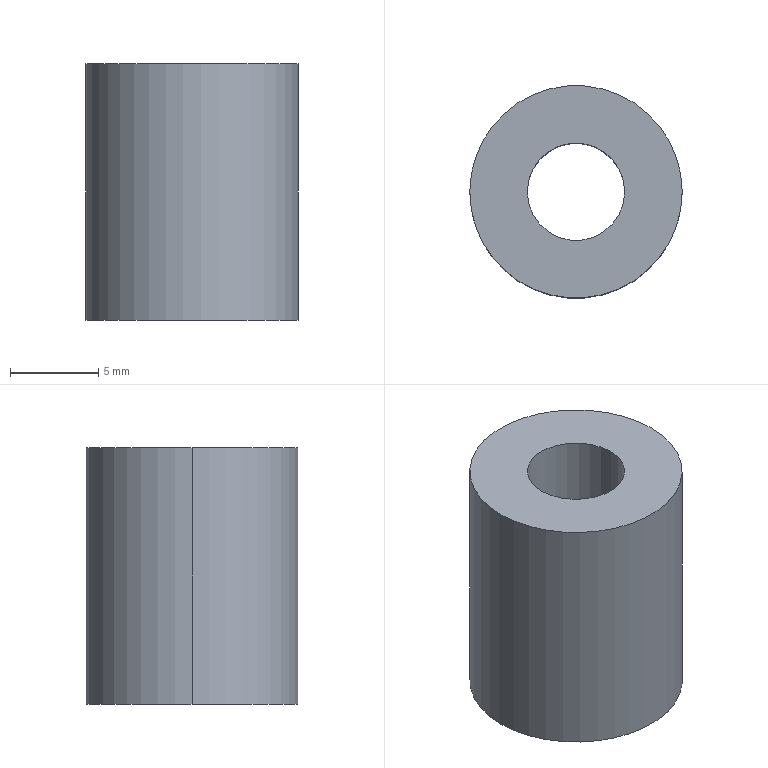Part | SolidWorks | features BaseBody 1 | 1 solid | 6 faces | box 12 x 12 x 14.5 mm | volume 1295 mm3 | cylinder 4 | plane 2 | commonest cylinder face diameters 5.5 x2 12 x2
STEP:
#1=CARTESIAN_POINT('',(213.479,1868.544,-23.5));
#2=VERTEX_POINT('',#1);
#3=CARTESIAN_POINT('',(201.479,1868.544,-23.5));
#4=VERTEX_POINT('',#3);
#5=CARTESIAN_POINT('',(207.479,1868.544,-23.5));
#6=DIRECTION('',(0.,0.,1.));
#7=DIRECTION('',(1.,0.,0.));
#8=AXIS2_PLACEMENT_3D('',#5,#6,#7);
#9=CIRCLE('',#8,6.);
#10=EDGE_CURVE('',#2,#4,#9,.T.);
#11=ORIENTED_EDGE('',*,*,#10,.T.);
#12=CARTESIAN_POINT('',(201.479,1868.544,-9.));
#13=VERTEX_POINT('',#12);
#14=CARTESIAN_POINT('',(201.479,1868.544,-23.5));
#15=DIRECTION('',(0.,0.,1.));
#16=VECTOR('',#15,1000.);
#17=LINE('',#14,#16);
#18=EDGE_CURVE('',#4,#13,#17,.T.);
#19=ORIENTED_EDGE('',*,*,#18,.T.);
#20=CARTESIAN_POINT('',(213.479,1868.544,-9.));
#21=VERTEX_POINT('',#20);
#22=CARTESIAN_POINT('',(207.479,1868.544,-9.));
#23=DIRECTION('',(0.,0.,-1.));
#24=DIRECTION('',(1.,0.,0.));
#25=AXIS2_PLACEMENT_3D('',#22,#23,#24);
#26=CIRCLE('',#25,6.);
#27=EDGE_CURVE('',#13,#21,#26,.T.);
#28=ORIENTED_EDGE('',*,*,#27,.T.);
#29=CARTESIAN_POINT('',(213.479,1868.544,-23.5));
#30=DIRECTION('',(0.,0.,1.));
#31=VECTOR('',#30,1000.);
#32=LINE('',#29,#31);
#33=EDGE_CURVE('',#2,#21,#32,.T.);
#34=ORIENTED_EDGE('',*,*,#33,.F.);
#35=EDGE_LOOP('',(#11,#19,#28,#34));
#36=FACE_OUTER_BOUND('',#35,.T.);
#37=CARTESIAN_POINT('',(207.479,1868.544,-23.5));
#38=DIRECTION('',(0.,0.,1.));
#39=DIRECTION('',(1.,0.,0.));
#40=AXIS2_PLACEMENT_3D('',#37,#38,#39);
#41=CYLINDRICAL_SURFACE('',#40,6.);
#42=ADVANCED_FACE('',(#36),#41,.T.);
#43=CARTESIAN_POINT('',(204.729,1868.544,-23.5));
#44=VERTEX_POINT('',#43);
#45=CARTESIAN_POINT('',(210.229,1868.544,-23.5));
#46=VERTEX_POINT('',#45);
#47=CARTESIAN_POINT('',(207.479,1868.544,-23.5));
#48=DIRECTION('',(0.,0.,1.));
#49=DIRECTION('',(1.,0.,0.));
#50=AXIS2_PLACEMENT_3D('',#47,#48,#49);
#51=CIRCLE('',#50,2.75);
#52=EDGE_CURVE('',#44,#46,#51,.T.);
#53=ORIENTED_EDGE('',*,*,#52,.F.);
#54=CARTESIAN_POINT('',(204.729,1868.544,-9.));
#55=VERTEX_POINT('',#54);
#56=CARTESIAN_POINT('',(204.729,1868.544,-23.5));
#57=DIRECTION('',(0.,0.,1.));
#58=VECTOR('',#57,1000.);
#59=LINE('',#56,#58);
#60=EDGE_CURVE('',#44,#55,#59,.T.);
#61=ORIENTED_EDGE('',*,*,#60,.T.);
#62=CARTESIAN_POINT('',(210.229,1868.544,-9.));
#63=VERTEX_POINT('',#62);
#64=CARTESIAN_POINT('',(207.479,1868.544,-9.));
#65=DIRECTION('',(0.,0.,1.));
#66=DIRECTION('',(1.,0.,0.));
#67=AXIS2_PLACEMENT_3D('',#64,#65,#66);
#68=CIRCLE('',#67,2.75);
#69=EDGE_CURVE('',#55,#63,#68,.T.);
#70=ORIENTED_EDGE('',*,*,#69,.T.);
#71=CARTESIAN_POINT('',(210.229,1868.544,-23.5));
#72=DIRECTION('',(0.,0.,1.));
#73=VECTOR('',#72,1000.);
#74=LINE('',#71,#73);
#75=EDGE_CURVE('',#46,#63,#74,.T.);
#76=ORIENTED_EDGE('',*,*,#75,.F.);
#77=EDGE_LOOP('',(#53,#61,#70,#76));
#78=FACE_OUTER_BOUND('',#77,.T.);
#79=CARTESIAN_POINT('',(207.479,1868.544,-23.5));
#80=DIRECTION('',(0.,0.,1.));
#81=DIRECTION('',(1.,0.,0.));
#82=AXIS2_PLACEMENT_3D('',#79,#80,#81);
#83=CYLINDRICAL_SURFACE('',#82,2.75);
#84=ADVANCED_FACE('',(#78),#83,.F.);
#85=ORIENTED_EDGE('',*,*,#18,.F.);
#86=CARTESIAN_POINT('',(207.479,1868.544,-23.5));
#87=DIRECTION('',(0.,0.,1.));
#88=DIRECTION('',(1.,0.,0.));
#89=AXIS2_PLACEMENT_3D('',#86,#87,#88);
#90=CIRCLE('',#89,6.);
#91=EDGE_CURVE('',#4,#2,#90,.T.);
#92=ORIENTED_EDGE('',*,*,#91,.T.);
#93=ORIENTED_EDGE('',*,*,#33,.T.);
#94=CARTESIAN_POINT('',(207.479,1868.544,-9.));
#95=DIRECTION('',(0.,0.,-1.));
#96=DIRECTION('',(1.,0.,0.));
#97=AXIS2_PLACEMENT_3D('',#94,#95,#96);
#98=CIRCLE('',#97,6.);
#99=EDGE_CURVE('',#21,#13,#98,.T.);
#100=ORIENTED_EDGE('',*,*,#99,.T.);
#101=EDGE_LOOP('',(#85,#92,#93,#100));
#102=FACE_OUTER_BOUND('',#101,.T.);
#103=CARTESIAN_POINT('',(207.479,1868.544,-23.5));
#104=DIRECTION('',(0.,0.,1.));
#105=DIRECTION('',(1.,0.,0.));
#106=AXIS2_PLACEMENT_3D('',#103,#104,#105);
#107=CYLINDRICAL_SURFACE('',#106,6.);
#108=ADVANCED_FACE('',(#102),#107,.T.);
#109=CARTESIAN_POINT('',(207.479,1868.544,-23.5));
#110=DIRECTION('',(0.,0.,1.));
#111=DIRECTION('',(1.,0.,0.));
#112=AXIS2_PLACEMENT_3D('',#109,#110,#111);
#113=CIRCLE('',#112,2.75);
#114=EDGE_CURVE('',#46,#44,#113,.T.);
#115=ORIENTED_EDGE('',*,*,#114,.T.);
#116=ORIENTED_EDGE('',*,*,#52,.T.);
#117=EDGE_LOOP('',(#115,#116));
#118=FACE_BOUND('',#117,.T.);
#119=ORIENTED_EDGE('',*,*,#10,.F.);
#120=ORIENTED_EDGE('',*,*,#91,.F.);
#121=EDGE_LOOP('',(#119,#120));
#122=FACE_OUTER_BOUND('',#121,.T.);
#123=CARTESIAN_POINT('',(207.479,1868.544,-23.5));
#124=DIRECTION('',(0.,0.,-1.));
#125=DIRECTION('',(-1.,0.,0.));
#126=AXIS2_PLACEMENT_3D('',#123,#124,#125);
#127=PLANE('',#126);
#128=ADVANCED_FACE('',(#118,#122),#127,.T.);
#129=CARTESIAN_POINT('',(207.479,1868.544,-9.));
#130=DIRECTION('',(0.,0.,1.));
#131=DIRECTION('',(1.,0.,0.));
#132=AXIS2_PLACEMENT_3D('',#129,#130,#131);
#133=CIRCLE('',#132,2.75);
#134=EDGE_CURVE('',#63,#55,#133,.T.);
#135=ORIENTED_EDGE('',*,*,#134,.F.);
#136=ORIENTED_EDGE('',*,*,#69,.F.);
#137=EDGE_LOOP('',(#135,#136));
#138=FACE_BOUND('',#137,.T.);
#139=ORIENTED_EDGE('',*,*,#99,.F.);
#140=ORIENTED_EDGE('',*,*,#27,.F.);
#141=EDGE_LOOP('',(#139,#140));
#142=FACE_OUTER_BOUND('',#141,.T.);
#143=CARTESIAN_POINT('',(207.479,1868.544,-9.));
#144=DIRECTION('',(0.,0.,-1.));
#145=DIRECTION('',(-1.,0.,0.));
#146=AXIS2_PLACEMENT_3D('',#143,#144,#145);
#147=PLANE('',#146);
#148=ADVANCED_FACE('',(#138,#142),#147,.F.);
#149=ORIENTED_EDGE('',*,*,#60,.F.);
#150=ORIENTED_EDGE('',*,*,#114,.F.);
#151=ORIENTED_EDGE('',*,*,#75,.T.);
#152=ORIENTED_EDGE('',*,*,#134,.T.);
#153=EDGE_LOOP('',(#149,#150,#151,#152));
#154=FACE_OUTER_BOUND('',#153,.T.);
#155=CARTESIAN_POINT('',(207.479,1868.544,-23.5));
#156=DIRECTION('',(0.,0.,1.));
#157=DIRECTION('',(1.,0.,0.));
#158=AXIS2_PLACEMENT_3D('',#155,#156,#157);
#159=CYLINDRICAL_SURFACE('',#158,2.75);
#160=ADVANCED_FACE('',(#154),#159,.F.);
#161=CLOSED_SHELL('',(#42,#84,#108,#128,#148,#160));
#162=MANIFOLD_SOLID_BREP('',#161);
#163=CARTESIAN_POINT('',(0.,0.,0.));
#164=DIRECTION('',(0.,0.,1.));
#165=DIRECTION('',(1.,0.,0.));
#166=AXIS2_PLACEMENT_3D('',#163,#164,#165);
#167=(LENGTH_UNIT()NAMED_UNIT(*)SI_UNIT(.MILLI.,.METRE.));
#168=UNCERTAINTY_MEASURE_WITH_UNIT(LENGTH_MEASURE(0.00001),#167,'','');
#169=(NAMED_UNIT(*)PLANE_ANGLE_UNIT()SI_UNIT($,.RADIAN.));
#170=(NAMED_UNIT(*)SI_UNIT($,.STERADIAN.)SOLID_ANGLE_UNIT());
#171=(GEOMETRIC_REPRESENTATION_CONTEXT(3)GLOBAL_UNCERTAINTY_ASSIGNED_CONTEXT((#168))GLOBAL_UNIT_ASSIGNED_CONTEXT((#167,#169,#170))REPRESENTATION_CONTEXT('',''));
#172=ADVANCED_BREP_SHAPE_REPRESENTATION('',(#162,#166),#171);